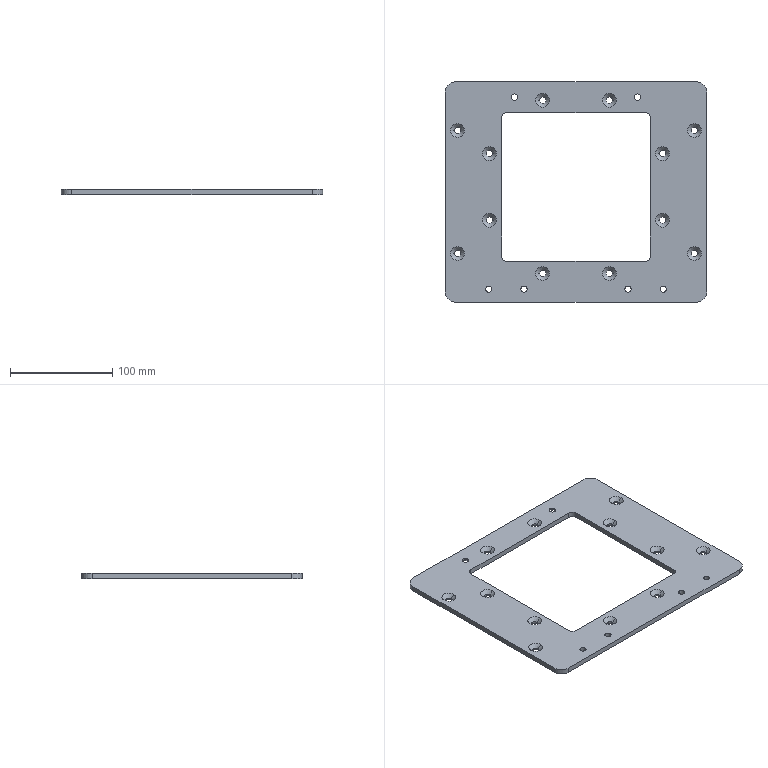NC program | NX | posted with a generic post | part box 255 x 215 x 5 mm
Lines 1 to 1055 of 7663:
N10 G17 G21 G94 G90
(DRILLING , TOOL : D6A45)
N12 T01 M6
N14 G54
N16 G17 G0 G90 X115.5 Y60. S5000 M3
N18 G43 Z30. H1
N20 G94 G81 G98 Z-1. F350. R3.
N22 X84.5 Y37.5
N24 X60. Y92.5
N26 X32.5 Y89.5
N28 X-32.5
N30 X-60. Y92.5
N32 X-115.5 Y60.
N34 X-84.5 Y37.5
N36 Y-27.5
N38 X-115.5 Y-60.
N40 X-85.25 Y-94.85
N42 X-50.75
N44 X-32.5 Y-79.5
N46 X32.5
N48 X50.75 Y-94.85
N50 X85.25
N52 X115.5 Y-60.
N54 X84.5 Y-27.5
N56 G80
N58 G0 X84.5 Y-27.5 Z30.
N60 M5
(DRILLING_COPY , TOOL : 6.5ZT)
N62 T10 M6
N64 G54
N66 G17 G0 G90 X115.5 Y-60. S2000 M3
N68 G43 Z30. H10
N70 G94 G83 G98 Z-8.453 F300. Q2. R3.
N72 X84.5 Y-27.5
N74 Y37.5
N76 X115.5 Y60.
N78 X60. Y92.5
N80 X32.5 Y89.5
N82 X-32.5
N84 X-60. Y92.5
N86 X-115.5 Y60.
N88 X-84.5 Y37.5
N90 Y-27.5
N92 X-115.5 Y-60.
N94 X-32.5 Y-79.5
N96 X32.5
N98 G80
N100 G0 X32.5 Y-79.5 Z30.
N102 M5
(DRILLING_COPY_1 , TOOL : 6.0ZT)
N104 T16 M6
N106 G54
N108 G17 G0 G90 X85.25 Y-94.85 S2000 M3
N110 G43 Z30. H16
N112 G94 G83 G98 Z-8.303 F250. Q2. R3.
N114 X50.75
N116 X-50.75
N118 X-85.25
N120 G80
N122 G0 X-85.25 Y-94.85 Z30.
N124 M5
(ZLEVEL_PROFILE_COPY_1 , TOOL : D10)
N126 T15 M6
N128 G54
N130 G17 G0 G90 X67.4 Y32.319 S9500 M3
N132 G43 Z30. H15
N134 Z1.5
N136 G94 G1 Y72.39 Z-0.6 F1000.
N138 X67.311 Y72.4 F2000.
N140 X-67.35
N142 X-67.4 Y72.39
N144 Y-62.311
N146 X-67.39 Y-62.4
N148 X67.39
N150 X67.4 Y-62.311
N152 Y72.39
N154 X62.546 Y72.4 Z-0.605
N156 X-57.732 Z-0.739
N158 X-62.541 Z-0.745
N160 X-67.349 Y72.392 Z-0.75
N162 X-67.386 Y72.387
N164 X-67.39 Y72.357
N166 X-67.4 Y67.567 Z-0.755
N168 Y62.768 Z-0.761
N170 Y-52.689 Z-0.889
N172 Y-57.5 Z-0.895
N174 X-67.396 Y-62.31 Z-0.9
N176 X-67.388 Y-62.385
N178 X-67.327 Y-62.393
N180 X-62.548 Y-62.4 Z-0.905
N182 X-57.762 Z-0.911
N184 X57.762 Z-1.039
N186 X62.548 Z-1.045
N188 X67.327 Y-62.393 Z-1.05
N190 X67.388 Y-62.385
N192 X67.396 Y-62.31
N194 X67.4 Y-57.5 Z-1.055
N196 Y-52.689 Z-1.061
N198 Y67.579 Z-1.195
N200 Y72.39 Z-1.2
N202 X62.546 Y72.4 Z-1.205
N204 X-57.732 Z-1.339
N206 X-62.541 Z-1.345
N208 X-67.349 Y72.392 Z-1.35
N210 X-67.386 Y72.387
N212 X-67.39 Y72.357
N214 X-67.4 Y67.567 Z-1.355
N216 Y62.768 Z-1.361
N218 Y-52.689 Z-1.489
N220 Y-57.5 Z-1.495
N222 X-67.396 Y-62.31 Z-1.5
N224 X-67.388 Y-62.385
N226 X-67.327 Y-62.393
N228 X-62.548 Y-62.4 Z-1.505
N230 X-57.762 Z-1.511
N232 X57.762 Z-1.639
N234 X62.548 Z-1.645
N236 X67.327 Y-62.393 Z-1.65
N238 X67.388 Y-62.385
N240 X67.396 Y-62.31
N242 X67.4 Y-57.5 Z-1.655
N244 Y-52.689 Z-1.661
N246 Y67.579 Z-1.795
N248 Y72.389 Z-1.8
N250 X62.546 Y72.4 Z-1.805
N252 X-57.732 Z-1.939
N254 X-62.54 Z-1.945
N256 X-67.349 Y72.392 Z-1.95
N258 X-67.386 Y72.387
N260 X-67.39 Y72.357
N262 X-67.4 Y67.567 Z-1.955
N264 Y62.768 Z-1.961
N266 Y-52.689 Z-2.089
N268 Y-57.5 Z-2.095
N270 X-67.396 Y-62.31 Z-2.1
N272 X-67.388 Y-62.384
N274 X-67.328 Y-62.393
N276 X-62.548 Y-62.4 Z-2.105
N278 X-57.762 Z-2.111
N280 X57.762 Z-2.239
N282 X62.548 Z-2.245
N284 X67.328 Y-62.393 Z-2.25
N286 X67.388 Y-62.384
N288 X67.396 Y-62.31
N290 X67.4 Y-57.5 Z-2.255
N292 Y-52.689 Z-2.261
N294 Y67.579 Z-2.395
N296 Y72.389 Z-2.4
N298 X62.546 Y72.4 Z-2.405
N300 X-57.732 Z-2.539
N302 X-62.54 Z-2.545
N304 X-67.349 Y72.392 Z-2.55
N306 X-67.386 Y72.388
N308 X-67.39 Y72.355
N310 X-67.4 Y67.566 Z-2.555
N312 Y62.768 Z-2.561
N314 Y-52.689 Z-2.689
N316 Y-57.5 Z-2.695
N318 X-67.396 Y-62.31 Z-2.7
N320 X-67.388 Y-62.384
N322 X-67.328 Y-62.393
N324 X-62.548 Y-62.4 Z-2.705
N326 X-57.762 Z-2.711
N328 X57.762 Z-2.839
N330 X62.548 Z-2.845
N332 X67.328 Y-62.393 Z-2.85
N334 X67.388 Y-62.384
N336 X67.396 Y-62.31
N338 X67.4 Y-57.5 Z-2.855
N340 Y-52.689 Z-2.861
N342 Y67.579 Z-2.995
N344 Y72.389 Z-3.
N346 X62.546 Y72.4 Z-3.005
N348 X-57.732 Z-3.139
N350 X-62.54 Z-3.145
N352 X-67.349 Y72.392 Z-3.15
N354 X-67.386 Y72.388
N356 X-67.39 Y72.355
N358 X-67.4 Y67.566 Z-3.155
N360 Y62.768 Z-3.161
N362 Y-52.689 Z-3.289
N364 Y-57.5 Z-3.295
N366 X-67.396 Y-62.31 Z-3.3
N368 X-67.388 Y-62.384
N370 X-67.328 Y-62.393
N372 X-62.548 Y-62.4 Z-3.305
N374 X-57.762 Z-3.311
N376 X57.762 Z-3.439
N378 X62.548 Z-3.445
N380 X67.328 Y-62.393 Z-3.45
N382 X67.388 Y-62.384
N384 X67.396 Y-62.31
N386 X67.4 Y-57.5 Z-3.455
N388 Y-52.689 Z-3.461
N390 Y67.579 Z-3.595
N392 Y72.389 Z-3.6
N394 X62.546 Y72.4 Z-3.605
N396 X-57.732 Z-3.739
N398 X-62.54 Z-3.745
N400 X-67.348 Y72.392 Z-3.75
N402 X-67.386 Y72.388
N404 X-67.39 Y72.355
N406 X-67.4 Y67.566 Z-3.755
N408 Y62.768 Z-3.761
N410 Y-52.689 Z-3.889
N412 Y-57.5 Z-3.895
N414 X-67.396 Y-62.31 Z-3.9
N416 X-67.388 Y-62.384
N418 X-67.328 Y-62.393
N420 X-62.548 Y-62.4 Z-3.905
N422 X-57.762 Z-3.911
N424 X57.762 Z-4.039
N426 X62.548 Z-4.045
N428 X67.328 Y-62.393 Z-4.05
N430 X67.388 Y-62.384
N432 X67.396 Y-62.31
N434 X67.4 Y-57.5 Z-4.055
N436 Y-52.689 Z-4.061
N438 Y67.579 Z-4.195
N440 Y72.389 Z-4.2
N442 X62.546 Y72.4 Z-4.205
N444 X-57.732 Z-4.339
N446 X-62.54 Z-4.345
N448 X-67.348 Y72.392 Z-4.35
N450 X-67.386 Y72.388
N452 X-67.39 Y72.355
N454 X-67.4 Y67.566 Z-4.355
N456 Y62.768 Z-4.361
N458 Y-52.689 Z-4.489
N460 Y-57.5 Z-4.495
N462 X-67.396 Y-62.31 Z-4.5
N464 X-67.388 Y-62.384
N466 X-67.328 Y-62.393
N468 X-62.548 Y-62.4 Z-4.505
N470 X-57.762 Z-4.511
N472 X57.762 Z-4.639
N474 X62.548 Z-4.645
N476 X67.328 Y-62.393 Z-4.65
N478 X67.388 Y-62.384
N480 X67.396 Y-62.31
N482 X67.4 Y-57.5 Z-4.655
N484 Y-52.689 Z-4.661
N486 Y67.579 Z-4.795
N488 Y72.389 Z-4.8
N490 X67.311 Y72.4
N492 X-67.35
N494 X-67.4 Y72.39
N496 Y-62.311
N498 X-67.389 Y-62.4
N500 X67.389
N502 X67.4 Y-62.311
N504 Y72.389
N506 Z-3.3
N508 G0 Z30.
(ZLEVEL_PROFILE_COPY_1_COPY , TOOL : D10)
N510 X-132.6 Y82.125
N512 Z1.5
N514 G1 Y98.452 Z0.644 F1000.
N516 X-132.254 Y100.854 Z0.517
N518 X-131.528 Y103.169 Z0.39
N520 X-130.441 Y105.338 Z0.263
N522 X-129.022 Y107.306 Z0.136
N524 X-127.306 Y109.022 Z0.009
N526 X-125.338 Y110.441 Z-0.119
N528 X-123.169 Y111.528 Z-0.246
N530 X-120.854 Y112.254 Z-0.373
N532 X-118.452 Y112.6 Z-0.5
N534 X-117.5 Z-0.55
N536 X117.5 F2000.
N538 G2 X132.6 Y97.5 R15.1
N540 G1 Y-97.5
N542 G2 X117.5 Y-112.6 R15.1
N544 G1 X-117.5
N546 G2 X-132.6 Y-97.5 R15.1
N548 G1 Y97.5
N550 G2 X-117.5 Y112.6 R15.1
N552 G1 X117.5 Z-0.685
N554 X118.412 Y112.572 Z-0.686
N556 X119.32 Y112.49
N558 X120.222 Y112.353 Z-0.687
N560 X121.114 Y112.161
N562 X121.992 Y111.916 Z-0.688
N564 X122.855 Y111.619 Z-0.689
N566 X123.697 Y111.27
N568 X124.517 Y110.87 Z-0.69
N570 X125.312 Y110.422
N572 X126.078 Y109.927 Z-0.691
N574 X126.812 Y109.386
N576 X127.513 Y108.803 Z-0.692
N578 X128.177 Y108.177
N580 X128.803 Y107.513 Z-0.693
N582 X129.386 Y106.812
N584 X129.927 Y106.078 Z-0.694
N586 X130.422 Y105.312
N588 X130.87 Y104.517 Z-0.695
N590 X131.27 Y103.697
N592 X131.619 Y102.855 Z-0.696
N594 X131.916 Y101.992
N596 X132.161 Y101.114 Z-0.697
N598 X132.353 Y100.222
N600 X132.49 Y99.32 Z-0.698
N602 X132.572 Y98.412
N604 X132.6 Y97.5 Z-0.699
N606 Y-97.5 Z-0.811
N608 X132.572 Y-98.412 Z-0.812
N610 X132.49 Y-99.32
N612 X132.353 Y-100.222 Z-0.813
N614 X132.161 Y-101.114
N616 X131.916 Y-101.992 Z-0.814
N618 X131.619 Y-102.855
N620 X131.27 Y-103.697 Z-0.815
N622 X130.87 Y-104.517 Z-0.816
N624 X130.422 Y-105.312
N626 X129.927 Y-106.078 Z-0.817
N628 X129.386 Y-106.812
N630 X128.803 Y-107.513 Z-0.818
N632 X128.177 Y-108.177
N634 X127.513 Y-108.803 Z-0.819
N636 X126.812 Y-109.386
N638 X126.078 Y-109.927 Z-0.82
N640 X125.312 Y-110.422
N642 X124.517 Y-110.87 Z-0.821
N644 X123.697 Y-111.27
N646 X122.855 Y-111.619 Z-0.822
N648 X121.992 Y-111.916
N650 X121.114 Y-112.161 Z-0.823
N652 X120.222 Y-112.353
N654 X119.32 Y-112.49 Z-0.824
N656 X118.412 Y-112.572
N658 X117.5 Y-112.6 Z-0.825
N660 X-117.5 Z-0.96
N662 X-118.412 Y-112.572 Z-0.961
N664 X-119.32 Y-112.49
N666 X-120.222 Y-112.353 Z-0.962
N668 X-121.114 Y-112.161
N670 X-121.992 Y-111.916 Z-0.963
N672 X-122.855 Y-111.619 Z-0.964
N674 X-123.697 Y-111.27
N676 X-124.517 Y-110.87 Z-0.965
N678 X-125.312 Y-110.422
N680 X-126.078 Y-109.927 Z-0.966
N682 X-126.812 Y-109.386
N684 X-127.513 Y-108.803 Z-0.967
N686 X-128.177 Y-108.177
N688 X-128.803 Y-107.513 Z-0.968
N690 X-129.386 Y-106.812
N692 X-129.927 Y-106.078 Z-0.969
N694 X-130.422 Y-105.312
N696 X-130.87 Y-104.517 Z-0.97
N698 X-131.27 Y-103.697
N700 X-131.619 Y-102.855 Z-0.971
N702 X-131.916 Y-101.992
N704 X-132.161 Y-101.114 Z-0.972
N706 X-132.353 Y-100.222
N708 X-132.49 Y-99.32 Z-0.973
N710 X-132.572 Y-98.412
N712 X-132.6 Y-97.5 Z-0.974
N714 Y97.5 Z-1.086
N716 X-132.572 Y98.412 Z-1.087
N718 X-132.49 Y99.32
N720 X-132.353 Y100.222 Z-1.088
N722 X-132.161 Y101.114
N724 X-131.916 Y101.992 Z-1.089
N726 X-131.619 Y102.855
N728 X-131.27 Y103.697 Z-1.09
N730 X-130.87 Y104.517 Z-1.091
N732 X-130.422 Y105.312
N734 X-129.927 Y106.078 Z-1.092
N736 X-129.386 Y106.812
N738 X-128.803 Y107.513 Z-1.093
N740 X-128.177 Y108.177
N742 X-127.513 Y108.803 Z-1.094
N744 X-126.812 Y109.386
N746 X-126.078 Y109.927 Z-1.095
N748 X-125.312 Y110.422
N750 X-124.517 Y110.87 Z-1.096
N752 X-123.697 Y111.27
N754 X-122.855 Y111.619 Z-1.097
N756 X-121.992 Y111.916
N758 X-121.114 Y112.161 Z-1.098
N760 X-120.222 Y112.353
N762 X-119.32 Y112.49 Z-1.099
N764 X-118.412 Y112.572
N766 X-117.5 Y112.6 Z-1.1
N768 X117.5 Z-1.235
N770 X118.412 Y112.572 Z-1.236
N772 X119.32 Y112.49
N774 X120.222 Y112.353 Z-1.237
N776 X121.114 Y112.161
N778 X121.992 Y111.916 Z-1.238
N780 X122.855 Y111.619 Z-1.239
N782 X123.697 Y111.27
N784 X124.517 Y110.87 Z-1.24
N786 X125.312 Y110.422
N788 X126.078 Y109.927 Z-1.241
N790 X126.812 Y109.386
N792 X127.513 Y108.803 Z-1.242
N794 X128.177 Y108.177
N796 X128.803 Y107.513 Z-1.243
N798 X129.386 Y106.812
N800 X129.927 Y106.078 Z-1.244
N802 X130.422 Y105.312
N804 X130.87 Y104.517 Z-1.245
N806 X131.27 Y103.697
N808 X131.619 Y102.855 Z-1.246
N810 X131.916 Y101.992
N812 X132.161 Y101.114 Z-1.247
N814 X132.353 Y100.222
N816 X132.49 Y99.32 Z-1.248
N818 X132.572 Y98.412
N820 X132.6 Y97.5 Z-1.249
N822 Y-97.5 Z-1.361
N824 X132.572 Y-98.412 Z-1.362
N826 X132.49 Y-99.32
N828 X132.353 Y-100.222 Z-1.363
N830 X132.161 Y-101.114
N832 X131.916 Y-101.992 Z-1.364
N834 X131.619 Y-102.855
N836 X131.27 Y-103.697 Z-1.365
N838 X130.87 Y-104.517 Z-1.366
N840 X130.422 Y-105.312
N842 X129.927 Y-106.078 Z-1.367
N844 X129.386 Y-106.812
N846 X128.803 Y-107.513 Z-1.368
N848 X128.177 Y-108.177
N850 X127.513 Y-108.803 Z-1.369
N852 X126.812 Y-109.386
N854 X126.078 Y-109.927 Z-1.37
N856 X125.312 Y-110.422
N858 X124.517 Y-110.87 Z-1.371
N860 X123.697 Y-111.27
N862 X122.855 Y-111.619 Z-1.372
N864 X121.992 Y-111.916
N866 X121.114 Y-112.161 Z-1.373
N868 X120.222 Y-112.353
N870 X119.32 Y-112.49 Z-1.374
N872 X118.412 Y-112.572
N874 X117.5 Y-112.6 Z-1.375
N876 X-117.5 Z-1.51
N878 X-118.412 Y-112.572 Z-1.511
N880 X-119.32 Y-112.49
N882 X-120.222 Y-112.353 Z-1.512
N884 X-121.114 Y-112.161
N886 X-121.992 Y-111.916 Z-1.513
N888 X-122.855 Y-111.619 Z-1.514
N890 X-123.697 Y-111.27
N892 X-124.517 Y-110.87 Z-1.515
N894 X-125.312 Y-110.422
N896 X-126.078 Y-109.927 Z-1.516
N898 X-126.812 Y-109.386
N900 X-127.513 Y-108.803 Z-1.517
N902 X-128.177 Y-108.177
N904 X-128.803 Y-107.513 Z-1.518
N906 X-129.386 Y-106.812
N908 X-129.927 Y-106.078 Z-1.519
N910 X-130.422 Y-105.312
N912 X-130.87 Y-104.517 Z-1.52
N914 X-131.27 Y-103.697
N916 X-131.619 Y-102.855 Z-1.521
N918 X-131.916 Y-101.992
N920 X-132.161 Y-101.114 Z-1.522
N922 X-132.353 Y-100.222
N924 X-132.49 Y-99.32 Z-1.523
N926 X-132.572 Y-98.412
N928 X-132.6 Y-97.5 Z-1.524
N930 Y97.5 Z-1.636
N932 X-132.572 Y98.412 Z-1.637
N934 X-132.49 Y99.32
N936 X-132.353 Y100.222 Z-1.638
N938 X-132.161 Y101.114
N940 X-131.916 Y101.992 Z-1.639
N942 X-131.619 Y102.855
N944 X-131.27 Y103.697 Z-1.64
N946 X-130.87 Y104.517 Z-1.641
N948 X-130.422 Y105.312
N950 X-129.927 Y106.078 Z-1.642
N952 X-129.386 Y106.812
N954 X-128.803 Y107.513 Z-1.643
N956 X-128.177 Y108.177
N958 X-127.513 Y108.803 Z-1.644
N960 X-126.812 Y109.386
N962 X-126.078 Y109.927 Z-1.645
N964 X-125.312 Y110.422
N966 X-124.517 Y110.87 Z-1.646
N968 X-123.697 Y111.27
N970 X-122.855 Y111.619 Z-1.647
N972 X-121.992 Y111.916
N974 X-121.114 Y112.161 Z-1.648
N976 X-120.222 Y112.353
N978 X-119.32 Y112.49 Z-1.649
N980 X-118.412 Y112.572
N982 X-117.5 Y112.6 Z-1.65
N984 X117.5 Z-1.785
N986 X118.412 Y112.572 Z-1.786
N988 X119.32 Y112.49
N990 X120.222 Y112.353 Z-1.787
N992 X121.114 Y112.161
N994 X121.992 Y111.916 Z-1.788
N996 X122.855 Y111.619 Z-1.789
N998 X123.697 Y111.27
N1000 X124.517 Y110.87 Z-1.79
N1002 X125.312 Y110.422
N1004 X126.078 Y109.927 Z-1.791
N1006 X126.812 Y109.386
N1008 X127.513 Y108.803 Z-1.792
N1010 X128.177 Y108.177
N1012 X128.803 Y107.513 Z-1.793
N1014 X129.386 Y106.812
N1016 X129.927 Y106.078 Z-1.794
N1018 X130.422 Y105.312
N1020 X130.87 Y104.517 Z-1.795
N1022 X131.27 Y103.697
N1024 X131.619 Y102.855 Z-1.796
N1026 X131.916 Y101.992
N1028 X132.161 Y101.114 Z-1.797
N1030 X132.353 Y100.222
N1032 X132.49 Y99.32 Z-1.798
N1034 X132.572 Y98.412
N1036 X132.6 Y97.5 Z-1.799
N1038 Y-97.5 Z-1.911
N1040 X132.572 Y-98.412 Z-1.912
N1042 X132.49 Y-99.32
N1044 X132.353 Y-100.222 Z-1.913
N1046 X132.161 Y-101.114
N1048 X131.916 Y-101.992 Z-1.914
N1050 X131.619 Y-102.855
N1052 X131.27 Y-103.697 Z-1.915
N1054 X130.87 Y-104.517 Z-1.916
N1056 X130.422 Y-105.312
N1058 X129.927 Y-106.078 Z-1.917
N1060 X129.386 Y-106.812
N1062 X128.803 Y-107.513 Z-1.918
N1064 X128.177 Y-108.177
N1066 X127.513 Y-108.803 Z-1.919
N1068 X126.812 Y-109.386
N1070 X126.078 Y-109.927 Z-1.92
N1072 X125.312 Y-110.422
N1074 X124.517 Y-110.87 Z-1.921
N1076 X123.697 Y-111.27
N1078 X122.855 Y-111.619 Z-1.922
N1080 X121.992 Y-111.916
N1082 X121.114 Y-112.161 Z-1.923
N1084 X120.222 Y-112.353
N1086 X119.32 Y-112.49 Z-1.924
N1088 X118.412 Y-112.572
N1090 X117.5 Y-112.6 Z-1.925
N1092 X-117.5 Z-2.06
N1094 X-118.412 Y-112.572 Z-2.061
N1096 X-119.32 Y-112.49
N1098 X-120.222 Y-112.353 Z-2.062
N1100 X-121.114 Y-112.161
N1102 X-121.992 Y-111.916 Z-2.063
N1104 X-122.855 Y-111.619 Z-2.064
N1106 X-123.697 Y-111.27
N1108 X-124.517 Y-110.87 Z-2.065
N1110 X-125.312 Y-110.422
N1112 X-126.078 Y-109.927 Z-2.066
N1114 X-126.812 Y-109.386
N1116 X-127.513 Y-108.803 Z-2.067
N1118 X-128.177 Y-108.177
N1120 X-128.803 Y-107.513 Z-2.068
N1122 X-129.386 Y-106.812
N1124 X-129.927 Y-106.078 Z-2.069
N1126 X-130.422 Y-105.312
N1128 X-130.87 Y-104.517 Z-2.07
N1130 X-131.27 Y-103.697
N1132 X-131.619 Y-102.855 Z-2.071
N1134 X-131.916 Y-101.992
N1136 X-132.161 Y-101.114 Z-2.072
N1138 X-132.353 Y-100.222
N1140 X-132.49 Y-99.32 Z-2.073
N1142 X-132.572 Y-98.412
N1144 X-132.6 Y-97.5 Z-2.074
N1146 Y97.5 Z-2.186
N1148 X-132.572 Y98.412 Z-2.187
N1150 X-132.49 Y99.32
N1152 X-132.353 Y100.222 Z-2.188
N1154 X-132.161 Y101.114
N1156 X-131.916 Y101.992 Z-2.189
N1158 X-131.619 Y102.855
N1160 X-131.27 Y103.697 Z-2.19
N1162 X-130.87 Y104.517 Z-2.191
N1164 X-130.422 Y105.312
N1166 X-129.927 Y106.078 Z-2.192
N1168 X-129.386 Y106.812
N1170 X-128.803 Y107.513 Z-2.193
N1172 X-128.177 Y108.177
N1174 X-127.513 Y108.803 Z-2.194
N1176 X-126.812 Y109.386
N1178 X-126.078 Y109.927 Z-2.195
N1180 X-125.312 Y110.422
N1182 X-124.517 Y110.87 Z-2.196
N1184 X-123.697 Y111.27
N1186 X-122.855 Y111.619 Z-2.197
N1188 X-121.992 Y111.916
N1190 X-121.114 Y112.161 Z-2.198
N1192 X-120.222 Y112.353
N1194 X-119.32 Y112.49 Z-2.199
N1196 X-118.412 Y112.572
N1198 X-117.5 Y112.6 Z-2.2
N1200 X117.5 Z-2.335
N1202 X118.412 Y112.572 Z-2.336
N1204 X119.32 Y112.49
N1206 X120.222 Y112.353 Z-2.337
N1208 X121.114 Y112.161
N1210 X121.992 Y111.916 Z-2.338
N1212 X122.855 Y111.619 Z-2.339
N1214 X123.697 Y111.27
N1216 X124.517 Y110.87 Z-2.34
N1218 X125.312 Y110.422
N1220 X126.078 Y109.927 Z-2.341
N1222 X126.812 Y109.386
N1224 X127.513 Y108.803 Z-2.342
N1226 X128.177 Y108.177
N1228 X128.803 Y107.513 Z-2.343
N1230 X129.386 Y106.812
N1232 X129.927 Y106.078 Z-2.344
N1234 X130.422 Y105.312
N1236 X130.87 Y104.517 Z-2.345
N1238 X131.27 Y103.697
N1240 X131.619 Y102.855 Z-2.346
N1242 X131.916 Y101.992
N1244 X132.161 Y101.114 Z-2.347
N1246 X132.353 Y100.222
N1248 X132.49 Y99.32 Z-2.348
N1250 X132.572 Y98.412
N1252 X132.6 Y97.5 Z-2.349
N1254 Y-97.5 Z-2.461
N1256 X132.572 Y-98.412 Z-2.462
N1258 X132.49 Y-99.32
N1260 X132.353 Y-100.222 Z-2.463
N1262 X132.161 Y-101.114
N1264 X131.916 Y-101.992 Z-2.464
N1266 X131.619 Y-102.855
N1268 X131.27 Y-103.697 Z-2.465
N1270 X130.87 Y-104.517 Z-2.466
N1272 X130.422 Y-105.312
N1274 X129.927 Y-106.078 Z-2.467
N1276 X129.386 Y-106.812
N1278 X128.803 Y-107.513 Z-2.468
N1280 X128.177 Y-108.177
N1282 X127.513 Y-108.803 Z-2.469
N1284 X126.812 Y-109.386
N1286 X126.078 Y-109.927 Z-2.47
N1288 X125.312 Y-110.422
N1290 X124.517 Y-110.87 Z-2.471
N1292 X123.697 Y-111.27
N1294 X122.855 Y-111.619 Z-2.472
N1296 X121.992 Y-111.916
N1298 X121.114 Y-112.161 Z-2.473
N1300 X120.222 Y-112.353
N1302 X119.32 Y-112.49 Z-2.474
N1304 X118.412 Y-112.572
N1306 X117.5 Y-112.6 Z-2.475
N1308 X-117.5 Z-2.61
N1310 X-118.412 Y-112.572 Z-2.611
N1312 X-119.32 Y-112.49
N1314 X-120.222 Y-112.353 Z-2.612
N1316 X-121.114 Y-112.161
N1318 X-121.992 Y-111.916 Z-2.613
N1320 X-122.855 Y-111.619 Z-2.614
N1322 X-123.697 Y-111.27
N1324 X-124.517 Y-110.87 Z-2.615
N1326 X-125.312 Y-110.422
N1328 X-126.078 Y-109.927 Z-2.616
N1330 X-126.812 Y-109.386
N1332 X-127.513 Y-108.803 Z-2.617
N1334 X-128.177 Y-108.177
N1336 X-128.803 Y-107.513 Z-2.618
N1338 X-129.386 Y-106.812
N1340 X-129.927 Y-106.078 Z-2.619
N1342 X-130.422 Y-105.312
N1344 X-130.87 Y-104.517 Z-2.62
N1346 X-131.27 Y-103.697
N1348 X-131.619 Y-102.855 Z-2.621
N1350 X-131.916 Y-101.992
N1352 X-132.161 Y-101.114 Z-2.622
N1354 X-132.353 Y-100.222
N1356 X-132.49 Y-99.32 Z-2.623
N1358 X-132.572 Y-98.412
N1360 X-132.6 Y-97.5 Z-2.624
N1362 Y97.5 Z-2.736
N1364 X-132.572 Y98.412 Z-2.737
N1366 X-132.49 Y99.32
N1368 X-132.353 Y100.222 Z-2.738
N1370 X-132.161 Y101.114
N1372 X-131.916 Y101.992 Z-2.739
N1374 X-131.619 Y102.855
N1376 X-131.27 Y103.697 Z-2.74
N1378 X-130.87 Y104.517 Z-2.741
N1380 X-130.422 Y105.312
N1382 X-129.927 Y106.078 Z-2.742
N1384 X-129.386 Y106.812
N1386 X-128.803 Y107.513 Z-2.743
N1388 X-128.177 Y108.177
N1390 X-127.513 Y108.803 Z-2.744
N1392 X-126.812 Y109.386
N1394 X-126.078 Y109.927 Z-2.745
N1396 X-125.312 Y110.422
N1398 X-124.517 Y110.87 Z-2.746
N1400 X-123.697 Y111.27
N1402 X-122.855 Y111.619 Z-2.747
N1404 X-121.992 Y111.916
N1406 X-121.114 Y112.161 Z-2.748
N1408 X-120.222 Y112.353
N1410 X-119.32 Y112.49 Z-2.749
N1412 X-118.412 Y112.572
N1414 X-117.5 Y112.6 Z-2.75
N1416 X117.5 Z-2.885
N1418 X118.412 Y112.572 Z-2.886
N1420 X119.32 Y112.49
N1422 X120.222 Y112.353 Z-2.887
N1424 X121.114 Y112.161
N1426 X121.992 Y111.916 Z-2.888
N1428 X122.855 Y111.619 Z-2.889
N1430 X123.697 Y111.27
N1432 X124.517 Y110.87 Z-2.89
N1434 X125.312 Y110.422
N1436 X126.078 Y109.927 Z-2.891
N1438 X126.812 Y109.386
N1440 X127.513 Y108.803 Z-2.892
N1442 X128.177 Y108.177
N1444 X128.803 Y107.513 Z-2.893
N1446 X129.386 Y106.812
N1448 X129.927 Y106.078 Z-2.894
N1450 X130.422 Y105.312
N1452 X130.87 Y104.517 Z-2.895
N1454 X131.27 Y103.697
N1456 X131.619 Y102.855 Z-2.896
N1458 X131.916 Y101.992
N1460 X132.161 Y101.114 Z-2.897
N1462 X132.353 Y100.222
N1464 X132.49 Y99.32 Z-2.898
N1466 X132.572 Y98.412
N1468 X132.6 Y97.5 Z-2.899
N1470 Y-97.5 Z-3.011
N1472 X132.572 Y-98.412 Z-3.012
N1474 X132.49 Y-99.32
N1476 X132.353 Y-100.222 Z-3.013
N1478 X132.161 Y-101.114
N1480 X131.916 Y-101.992 Z-3.014
N1482 X131.619 Y-102.855
N1484 X131.27 Y-103.697 Z-3.015
N1486 X130.87 Y-104.517 Z-3.016
N1488 X130.422 Y-105.312
N1490 X129.927 Y-106.078 Z-3.017
N1492 X129.386 Y-106.812
N1494 X128.803 Y-107.513 Z-3.018
N1496 X128.177 Y-108.177
N1498 X127.513 Y-108.803 Z-3.019
N1500 X126.812 Y-109.386
N1502 X126.078 Y-109.927 Z-3.02
N1504 X125.312 Y-110.422
N1506 X124.517 Y-110.87 Z-3.021
N1508 X123.697 Y-111.27
N1510 X122.855 Y-111.619 Z-3.022
N1512 X121.992 Y-111.916
N1514 X121.114 Y-112.161 Z-3.023
N1516 X120.222 Y-112.353
N1518 X119.32 Y-112.49 Z-3.024
N1520 X118.412 Y-112.572
N1522 X117.5 Y-112.6 Z-3.025
N1524 X-117.5 Z-3.16
N1526 X-118.412 Y-112.572 Z-3.161
N1528 X-119.32 Y-112.49
N1530 X-120.222 Y-112.353 Z-3.162
N1532 X-121.114 Y-112.161
N1534 X-121.992 Y-111.916 Z-3.163
N1536 X-122.855 Y-111.619 Z-3.164
N1538 X-123.697 Y-111.27
N1540 X-124.517 Y-110.87 Z-3.165
N1542 X-125.312 Y-110.422
N1544 X-126.078 Y-109.927 Z-3.166
N1546 X-126.812 Y-109.386
N1548 X-127.513 Y-108.803 Z-3.167
N1550 X-128.177 Y-108.177
N1552 X-128.803 Y-107.513 Z-3.168
N1554 X-129.386 Y-106.812
N1556 X-129.927 Y-106.078 Z-3.169
N1558 X-130.422 Y-105.312
N1560 X-130.87 Y-104.517 Z-3.17
N1562 X-131.27 Y-103.697
N1564 X-131.619 Y-102.855 Z-3.171
N1566 X-131.916 Y-101.992
N1568 X-132.161 Y-101.114 Z-3.172
N1570 X-132.353 Y-100.222
N1572 X-132.49 Y-99.32 Z-3.173
N1574 X-132.572 Y-98.412
N1576 X-132.6 Y-97.5 Z-3.174
N1578 Y97.5 Z-3.286
N1580 X-132.572 Y98.412 Z-3.287
N1582 X-132.49 Y99.32
N1584 X-132.353 Y100.222 Z-3.288
N1586 X-132.161 Y101.114
N1588 X-131.916 Y101.992 Z-3.289
N1590 X-131.619 Y102.855
N1592 X-131.27 Y103.697 Z-3.29
N1594 X-130.87 Y104.517 Z-3.291
N1596 X-130.422 Y105.312
N1598 X-129.927 Y106.078 Z-3.292
N1600 X-129.386 Y106.812
N1602 X-128.803 Y107.513 Z-3.293
N1604 X-128.177 Y108.177
N1606 X-127.513 Y108.803 Z-3.294
N1608 X-126.812 Y109.386
N1610 X-126.078 Y109.927 Z-3.295
N1612 X-125.312 Y110.422
N1614 X-124.517 Y110.87 Z-3.296
N1616 X-123.697 Y111.27
N1618 X-122.855 Y111.619 Z-3.297
N1620 X-121.992 Y111.916
N1622 X-121.114 Y112.161 Z-3.298
N1624 X-120.222 Y112.353
N1626 X-119.32 Y112.49 Z-3.299
N1628 X-118.412 Y112.572
N1630 X-117.5 Y112.6 Z-3.3
N1632 X117.5 Z-3.435
N1634 X118.412 Y112.572 Z-3.436
N1636 X119.32 Y112.49
N1638 X120.222 Y112.353 Z-3.437
N1640 X121.114 Y112.161
N1642 X121.992 Y111.916 Z-3.438
N1644 X122.855 Y111.619 Z-3.439
N1646 X123.697 Y111.27
N1648 X124.517 Y110.87 Z-3.44
N1650 X125.312 Y110.422
N1652 X126.078 Y109.927 Z-3.441
N1654 X126.812 Y109.386
N1656 X127.513 Y108.803 Z-3.442
N1658 X128.177 Y108.177
N1660 X128.803 Y107.513 Z-3.443
N1662 X129.386 Y106.812
N1664 X129.927 Y106.078 Z-3.444
N1666 X130.422 Y105.312
N1668 X130.87 Y104.517 Z-3.445
N1670 X131.27 Y103.697
N1672 X131.619 Y102.855 Z-3.446
N1674 X131.916 Y101.992
N1676 X132.161 Y101.114 Z-3.447
N1678 X132.353 Y100.222
N1680 X132.49 Y99.32 Z-3.448
N1682 X132.572 Y98.412
N1684 X132.6 Y97.5 Z-3.449
N1686 Y-97.5 Z-3.561
N1688 X132.572 Y-98.412 Z-3.562
N1690 X132.49 Y-99.32
N1692 X132.353 Y-100.222 Z-3.563
N1694 X132.161 Y-101.114
N1696 X131.916 Y-101.992 Z-3.564
N1698 X131.619 Y-102.855
N1700 X131.27 Y-103.697 Z-3.565
N1702 X130.87 Y-104.517 Z-3.566
N1704 X130.422 Y-105.312
N1706 X129.927 Y-106.078 Z-3.567
N1708 X129.386 Y-106.812
N1710 X128.803 Y-107.513 Z-3.568
N1712 X128.177 Y-108.177
N1714 X127.513 Y-108.803 Z-3.569
N1716 X126.812 Y-109.386
N1718 X126.078 Y-109.927 Z-3.57
N1720 X125.312 Y-110.422
N1722 X124.517 Y-110.87 Z-3.571
N1724 X123.697 Y-111.27
N1726 X122.855 Y-111.619 Z-3.572
N1728 X121.992 Y-111.916
N1730 X121.114 Y-112.161 Z-3.573
N1732 X120.222 Y-112.353
N1734 X119.32 Y-112.49 Z-3.574
N1736 X118.412 Y-112.572
N1738 X117.5 Y-112.6 Z-3.575
N1740 X-117.5 Z-3.71
N1742 X-118.412 Y-112.572 Z-3.711
N1744 X-119.32 Y-112.49
N1746 X-120.222 Y-112.353 Z-3.712
N1748 X-121.114 Y-112.161
N1750 X-121.992 Y-111.916 Z-3.713
N1752 X-122.855 Y-111.619 Z-3.714
N1754 X-123.697 Y-111.27
N1756 X-124.517 Y-110.87 Z-3.715
N1758 X-125.312 Y-110.422
N1760 X-126.078 Y-109.927 Z-3.716
N1762 X-126.812 Y-109.386
N1764 X-127.513 Y-108.803 Z-3.717
N1766 X-128.177 Y-108.177
N1768 X-128.803 Y-107.513 Z-3.718
N1770 X-129.386 Y-106.812
N1772 X-129.927 Y-106.078 Z-3.719
N1774 X-130.422 Y-105.312
N1776 X-130.87 Y-104.517 Z-3.72
N1778 X-131.27 Y-103.697
N1780 X-131.619 Y-102.855 Z-3.721
N1782 X-131.916 Y-101.992
N1784 X-132.161 Y-101.114 Z-3.722
N1786 X-132.353 Y-100.222
N1788 X-132.49 Y-99.32 Z-3.723
N1790 X-132.572 Y-98.412
N1792 X-132.6 Y-97.5 Z-3.724
N1794 Y97.5 Z-3.836
N1796 X-132.572 Y98.412 Z-3.837
N1798 X-132.49 Y99.32
N1800 X-132.353 Y100.222 Z-3.838
N1802 X-132.161 Y101.114
N1804 X-131.916 Y101.992 Z-3.839
N1806 X-131.619 Y102.855
N1808 X-131.27 Y103.697 Z-3.84
N1810 X-130.87 Y104.517 Z-3.841
N1812 X-130.422 Y105.312
N1814 X-129.927 Y106.078 Z-3.842
N1816 X-129.386 Y106.812
N1818 X-128.803 Y107.513 Z-3.843
N1820 X-128.177 Y108.177
N1822 X-127.513 Y108.803 Z-3.844
N1824 X-126.812 Y109.386
N1826 X-126.078 Y109.927 Z-3.845
N1828 X-125.312 Y110.422
N1830 X-124.517 Y110.87 Z-3.846
N1832 X-123.697 Y111.27
N1834 X-122.855 Y111.619 Z-3.847
N1836 X-121.992 Y111.916
N1838 X-121.114 Y112.161 Z-3.848
N1840 X-120.222 Y112.353
N1842 X-119.32 Y112.49 Z-3.849
N1844 X-118.412 Y112.572
N1846 X-117.5 Y112.6 Z-3.85
N1848 X117.5 Z-3.985
N1850 X118.412 Y112.572 Z-3.986
N1852 X119.32 Y112.49
N1854 X120.222 Y112.353 Z-3.987
N1856 X121.114 Y112.161
N1858 X121.992 Y111.916 Z-3.988
N1860 X122.855 Y111.619 Z-3.989
N1862 X123.697 Y111.27
N1864 X124.517 Y110.87 Z-3.99
N1866 X125.312 Y110.422
N1868 X126.078 Y109.927 Z-3.991
N1870 X126.812 Y109.386
N1872 X127.513 Y108.803 Z-3.992
N1874 X128.177 Y108.177
N1876 X128.803 Y107.513 Z-3.993
N1878 X129.386 Y106.812
N1880 X129.927 Y106.078 Z-3.994
N1882 X130.422 Y105.312
N1884 X130.87 Y104.517 Z-3.995
N1886 X131.27 Y103.697
N1888 X131.619 Y102.855 Z-3.996
N1890 X131.916 Y101.992
N1892 X132.161 Y101.114 Z-3.997
N1894 X132.353 Y100.222
N1896 X132.49 Y99.32 Z-3.998
N1898 X132.572 Y98.412
N1900 X132.6 Y97.5 Z-3.999
N1902 Y-97.5 Z-4.111
N1904 X132.572 Y-98.412 Z-4.112
N1906 X132.49 Y-99.32
N1908 X132.353 Y-100.222 Z-4.113
N1910 X132.161 Y-101.114
N1912 X131.916 Y-101.992 Z-4.114
N1914 X131.619 Y-102.855
N1916 X131.27 Y-103.697 Z-4.115
N1918 X130.87 Y-104.517 Z-4.116
N1920 X130.422 Y-105.312
N1922 X129.927 Y-106.078 Z-4.117
N1924 X129.386 Y-106.812
N1926 X128.803 Y-107.513 Z-4.118
N1928 X128.177 Y-108.177
N1930 X127.513 Y-108.803 Z-4.119
N1932 X126.812 Y-109.386
N1934 X126.078 Y-109.927 Z-4.12
N1936 X125.312 Y-110.422
N1938 X124.517 Y-110.87 Z-4.121
N1940 X123.697 Y-111.27
N1942 X122.855 Y-111.619 Z-4.122
N1944 X121.992 Y-111.916
N1946 X121.114 Y-112.161 Z-4.123
N1948 X120.222 Y-112.353
N1950 X119.32 Y-112.49 Z-4.124
N1952 X118.412 Y-112.572
N1954 X117.5 Y-112.6 Z-4.125
N1956 X-117.5 Z-4.26
N1958 X-118.412 Y-112.572 Z-4.261
N1960 X-119.32 Y-112.49
N1962 X-120.222 Y-112.353 Z-4.262
N1964 X-121.114 Y-112.161
N1966 X-121.992 Y-111.916 Z-4.263
N1968 X-122.855 Y-111.619 Z-4.264
N1970 X-123.697 Y-111.27
N1972 X-124.517 Y-110.87 Z-4.265
N1974 X-125.312 Y-110.422
N1976 X-126.078 Y-109.927 Z-4.266
N1978 X-126.812 Y-109.386
N1980 X-127.513 Y-108.803 Z-4.267
N1982 X-128.177 Y-108.177
N1984 X-128.803 Y-107.513 Z-4.268
N1986 X-129.386 Y-106.812
N1988 X-129.927 Y-106.078 Z-4.269
N1990 X-130.422 Y-105.312
N1992 X-130.87 Y-104.517 Z-4.27
N1994 X-131.27 Y-103.697
N1996 X-131.619 Y-102.855 Z-4.271
N1998 X-131.916 Y-101.992
N2000 X-132.161 Y-101.114 Z-4.272
N2002 X-132.353 Y-100.222
N2004 X-132.49 Y-99.32 Z-4.273
N2006 X-132.572 Y-98.412
N2008 X-132.6 Y-97.5 Z-4.274
N2010 Y97.5 Z-4.386
N2012 X-132.572 Y98.412 Z-4.387
N2014 X-132.49 Y99.32
N2016 X-132.353 Y100.222 Z-4.388
N2018 X-132.161 Y101.114
N2020 X-131.916 Y101.992 Z-4.389
N2022 X-131.619 Y102.855
N2024 X-131.27 Y103.697 Z-4.39
N2026 X-130.87 Y104.517 Z-4.391
N2028 X-130.422 Y105.312
N2030 X-129.927 Y106.078 Z-4.392
N2032 X-129.386 Y106.812
N2034 X-128.803 Y107.513 Z-4.393
N2036 X-128.177 Y108.177
N2038 X-127.513 Y108.803 Z-4.394
N2040 X-126.812 Y109.386
N2042 X-126.078 Y109.927 Z-4.395
N2044 X-125.312 Y110.422
N2046 X-124.517 Y110.87 Z-4.396
N2048 X-123.697 Y111.27
N2050 X-122.855 Y111.619 Z-4.397
N2052 X-121.992 Y111.916
N2054 X-121.114 Y112.161 Z-4.398
N2056 X-120.222 Y112.353
N2058 X-119.32 Y112.49 Z-4.399
N2060 X-118.412 Y112.572
N2062 X-117.5 Y112.6 Z-4.4
N2064 X117.5
N2066 G2 X132.6 Y97.5 R15.1
N2068 G1 Y-97.5
N2070 G2 X117.5 Y-112.6 R15.1
N2072 G1 X-117.5
N2074 G2 X-132.6 Y-97.5 R15.1
N2076 G1 Y97.5
N2078 G2 X-117.5 Y112.6 R15.1
N2080 G1 Z-2.9
N2082 G0 Z30.
N2084 M5